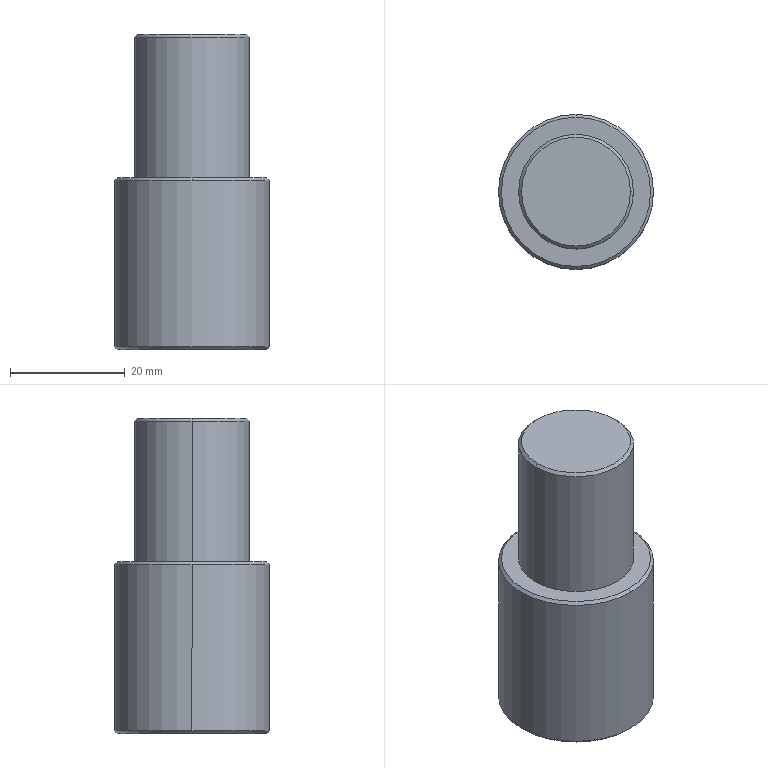Part | STEP file | Fixed head | 1 solid | 13 faces | box 27 x 27 x 55 mm | volume 25002 mm3 | cone 6 | cylinder 4 | plane 3 | commonest cylinder face diameters 20 x2 27 x2
STEP:
#1=CARTESIAN_POINT('',(0.,0.,0.));
#2=DIRECTION('',(0.,0.,1.));
#3=DIRECTION('',(1.,0.,0.));
#4=AXIS2_PLACEMENT_3D('',#1,#2,#3);
#5=CARTESIAN_POINT('',(0.,13.5,29.5));
#6=VERTEX_POINT('',#5);
#7=CARTESIAN_POINT('',(13.5,0.,29.5));
#8=VERTEX_POINT('',#7);
#9=CARTESIAN_POINT('',(0.,0.,29.5));
#10=DIRECTION('',(0.,0.,-1.));
#11=DIRECTION('',(-1.,0.,0.));
#12=AXIS2_PLACEMENT_3D('',#9,#10,#11);
#13=CIRCLE('',#12,13.5);
#14=CARTESIAN_POINT('',(0.,0.,30.));
#15=DIRECTION('',(0.,0.,-1.));
#16=DIRECTION('',(-1.,0.,0.));
#17=AXIS2_PLACEMENT_3D('',#14,#15,#16);
#18=CYLINDRICAL_SURFACE('',#17,13.5);
#19=CARTESIAN_POINT('',(0.,0.5));
#20=DIRECTION('',(1.,0.));
#21=VECTOR('',#20,1.);
#22=LINE('',#19,#21);
#23=(GEOMETRIC_REPRESENTATION_CONTEXT(2)PARAMETRIC_REPRESENTATION_CONTEXT()REPRESENTATION_CONTEXT('',''));
#24=DEFINITIONAL_REPRESENTATION('',(#22),#23);
#25=PCURVE('',#18,#24);
#26=CARTESIAN_POINT('',(0.,0.,29.5));
#27=DIRECTION('',(0.,0.,-1.));
#28=DIRECTION('',(0.,1.,0.));
#29=AXIS2_PLACEMENT_3D('',#26,#27,#28);
#30=CONICAL_SURFACE('',#29,13.5,0.7854);
#31=CARTESIAN_POINT('',(-1.571,0.));
#32=DIRECTION('',(1.,0.));
#33=VECTOR('',#32,1.);
#34=LINE('',#31,#33);
#35=(GEOMETRIC_REPRESENTATION_CONTEXT(2)PARAMETRIC_REPRESENTATION_CONTEXT()REPRESENTATION_CONTEXT('',''));
#36=DEFINITIONAL_REPRESENTATION('',(#34),#35);
#37=PCURVE('',#30,#36);
#38=SURFACE_CURVE('',#13,(#25,#37),.PCURVE_S1.);
#39=EDGE_CURVE('',#6,#8,#38,.T.);
#40=ORIENTED_EDGE('',*,*,#39,.T.);
#41=CARTESIAN_POINT('',(13.5,0.,0.5));
#42=VERTEX_POINT('',#41);
#43=CARTESIAN_POINT('',(13.5,0.,30.));
#44=DIRECTION('',(0.,0.,-1.));
#45=VECTOR('',#44,1.);
#46=LINE('',#43,#45);
#47=CARTESIAN_POINT('',(3.142,0.));
#48=DIRECTION('',(0.,1.));
#49=VECTOR('',#48,1.);
#50=LINE('',#47,#49);
#51=(GEOMETRIC_REPRESENTATION_CONTEXT(2)PARAMETRIC_REPRESENTATION_CONTEXT()REPRESENTATION_CONTEXT('',''));
#52=DEFINITIONAL_REPRESENTATION('',(#50),#51);
#53=PCURVE('',#18,#52);
#54=CARTESIAN_POINT('',(0.,0.,30.));
#55=DIRECTION('',(0.,0.,-1.));
#56=DIRECTION('',(-1.,0.,0.));
#57=AXIS2_PLACEMENT_3D('',#54,#55,#56);
#58=CYLINDRICAL_SURFACE('',#57,13.5);
#59=CARTESIAN_POINT('',(3.142,0.));
#60=DIRECTION('',(0.,1.));
#61=VECTOR('',#60,1.);
#62=LINE('',#59,#61);
#63=(GEOMETRIC_REPRESENTATION_CONTEXT(2)PARAMETRIC_REPRESENTATION_CONTEXT()REPRESENTATION_CONTEXT('',''));
#64=DEFINITIONAL_REPRESENTATION('',(#62),#63);
#65=PCURVE('',#58,#64);
#66=SURFACE_CURVE('',#46,(#53,#65),.PCURVE_S1.);
#67=EDGE_CURVE('',#8,#42,#66,.T.);
#68=ORIENTED_EDGE('',*,*,#67,.T.);
#69=CARTESIAN_POINT('',(-13.5,0.,0.5));
#70=VERTEX_POINT('',#69);
#71=CARTESIAN_POINT('',(0.,0.,0.5));
#72=DIRECTION('',(0.,0.,1.));
#73=DIRECTION('',(-1.,0.,0.));
#74=AXIS2_PLACEMENT_3D('',#71,#72,#73);
#75=CIRCLE('',#74,13.5);
#76=CARTESIAN_POINT('',(6.283,29.5));
#77=DIRECTION('',(-1.,0.));
#78=VECTOR('',#77,1.);
#79=LINE('',#76,#78);
#80=(GEOMETRIC_REPRESENTATION_CONTEXT(2)PARAMETRIC_REPRESENTATION_CONTEXT()REPRESENTATION_CONTEXT('',''));
#81=DEFINITIONAL_REPRESENTATION('',(#79),#80);
#82=PCURVE('',#18,#81);
#83=CARTESIAN_POINT('',(0.,0.,0.5));
#84=DIRECTION('',(0.,0.,1.));
#85=DIRECTION('',(1.,0.,0.));
#86=AXIS2_PLACEMENT_3D('',#83,#84,#85);
#87=CONICAL_SURFACE('',#86,13.5,0.7854);
#88=CARTESIAN_POINT('',(-3.142,0.));
#89=DIRECTION('',(1.,0.));
#90=VECTOR('',#89,1.);
#91=LINE('',#88,#90);
#92=(GEOMETRIC_REPRESENTATION_CONTEXT(2)PARAMETRIC_REPRESENTATION_CONTEXT()REPRESENTATION_CONTEXT('',''));
#93=DEFINITIONAL_REPRESENTATION('',(#91),#92);
#94=PCURVE('',#87,#93);
#95=SURFACE_CURVE('',#75,(#82,#94),.PCURVE_S1.);
#96=EDGE_CURVE('',#42,#70,#95,.T.);
#97=ORIENTED_EDGE('',*,*,#96,.T.);
#98=CARTESIAN_POINT('',(-13.5,0.,29.5));
#99=VERTEX_POINT('',#98);
#100=CARTESIAN_POINT('',(-13.5,0.,30.));
#101=DIRECTION('',(0.,0.,-1.));
#102=VECTOR('',#101,1.);
#103=LINE('',#100,#102);
#104=CARTESIAN_POINT('',(0.,0.));
#105=DIRECTION('',(0.,1.));
#106=VECTOR('',#105,1.);
#107=LINE('',#104,#106);
#108=(GEOMETRIC_REPRESENTATION_CONTEXT(2)PARAMETRIC_REPRESENTATION_CONTEXT()REPRESENTATION_CONTEXT('',''));
#109=DEFINITIONAL_REPRESENTATION('',(#107),#108);
#110=PCURVE('',#18,#109);
#111=CARTESIAN_POINT('',(6.283,0.));
#112=DIRECTION('',(0.,1.));
#113=VECTOR('',#112,1.);
#114=LINE('',#111,#113);
#115=(GEOMETRIC_REPRESENTATION_CONTEXT(2)PARAMETRIC_REPRESENTATION_CONTEXT()REPRESENTATION_CONTEXT('',''));
#116=DEFINITIONAL_REPRESENTATION('',(#114),#115);
#117=PCURVE('',#58,#116);
#118=SURFACE_CURVE('',#103,(#110,#117),.PCURVE_S1.);
#119=EDGE_CURVE('',#99,#70,#118,.T.);
#120=ORIENTED_EDGE('',*,*,#119,.F.);
#121=CARTESIAN_POINT('',(0.,0.,29.5));
#122=DIRECTION('',(0.,0.,-1.));
#123=DIRECTION('',(-1.,0.,0.));
#124=AXIS2_PLACEMENT_3D('',#121,#122,#123);
#125=CIRCLE('',#124,13.5);
#126=CARTESIAN_POINT('',(0.,0.5));
#127=DIRECTION('',(1.,0.));
#128=VECTOR('',#127,1.);
#129=LINE('',#126,#128);
#130=(GEOMETRIC_REPRESENTATION_CONTEXT(2)PARAMETRIC_REPRESENTATION_CONTEXT()REPRESENTATION_CONTEXT('',''));
#131=DEFINITIONAL_REPRESENTATION('',(#129),#130);
#132=PCURVE('',#18,#131);
#133=CARTESIAN_POINT('',(0.,0.,29.5));
#134=DIRECTION('',(0.,0.,-1.));
#135=DIRECTION('',(0.,1.,0.));
#136=AXIS2_PLACEMENT_3D('',#133,#134,#135);
#137=CONICAL_SURFACE('',#136,13.5,0.7854);
#138=CARTESIAN_POINT('',(4.712,0.));
#139=DIRECTION('',(1.,0.));
#140=VECTOR('',#139,1.);
#141=LINE('',#138,#140);
#142=(GEOMETRIC_REPRESENTATION_CONTEXT(2)PARAMETRIC_REPRESENTATION_CONTEXT()REPRESENTATION_CONTEXT('',''));
#143=DEFINITIONAL_REPRESENTATION('',(#141),#142);
#144=PCURVE('',#137,#143);
#145=SURFACE_CURVE('',#125,(#132,#144),.PCURVE_S1.);
#146=EDGE_CURVE('',#99,#6,#145,.T.);
#147=ORIENTED_EDGE('',*,*,#146,.T.);
#148=EDGE_LOOP('',(#40,#68,#97,#120,#147));
#149=FACE_BOUND('',#148,.T.);
#150=ADVANCED_FACE('',(#149),#18,.T.);
#151=CARTESIAN_POINT('',(13.,0.,0.));
#152=VERTEX_POINT('',#151);
#153=CARTESIAN_POINT('',(-13.,0.,0.));
#154=VERTEX_POINT('',#153);
#155=CARTESIAN_POINT('',(0.,0.,0.));
#156=DIRECTION('',(0.,0.,1.));
#157=DIRECTION('',(1.,0.,0.));
#158=AXIS2_PLACEMENT_3D('',#155,#156,#157);
#159=CIRCLE('',#158,13.);
#160=CARTESIAN_POINT('',(0.,-0.5));
#161=DIRECTION('',(1.,0.));
#162=VECTOR('',#161,1.);
#163=LINE('',#160,#162);
#164=(GEOMETRIC_REPRESENTATION_CONTEXT(2)PARAMETRIC_REPRESENTATION_CONTEXT()REPRESENTATION_CONTEXT('',''));
#165=DEFINITIONAL_REPRESENTATION('',(#163),#164);
#166=PCURVE('',#87,#165);
#167=CARTESIAN_POINT('',(0.,0.,0.));
#168=DIRECTION('',(0.,0.,1.));
#169=DIRECTION('',(1.,0.,0.));
#170=AXIS2_PLACEMENT_3D('',#167,#168,#169);
#171=PLANE('',#170);
#172=CARTESIAN_POINT('',(0.,0.));
#173=DIRECTION('',(1.,0.));
#174=AXIS2_PLACEMENT_2D('',#172,#173);
#175=CIRCLE('',#174,13.);
#176=(GEOMETRIC_REPRESENTATION_CONTEXT(2)PARAMETRIC_REPRESENTATION_CONTEXT()REPRESENTATION_CONTEXT('',''));
#177=DEFINITIONAL_REPRESENTATION('',(#175),#176);
#178=PCURVE('',#171,#177);
#179=SURFACE_CURVE('',#159,(#166,#178),.PCURVE_S1.);
#180=EDGE_CURVE('',#152,#154,#179,.T.);
#181=ORIENTED_EDGE('',*,*,#180,.T.);
#182=CARTESIAN_POINT('',(-13.5,0.,0.5));
#183=DIRECTION('',(-0.7071,0.,0.7071));
#184=VECTOR('',#183,1.);
#185=LINE('',#182,#184);
#186=CARTESIAN_POINT('',(3.142,0.));
#187=DIRECTION('',(0.,1.));
#188=VECTOR('',#187,1.);
#189=LINE('',#186,#188);
#190=(GEOMETRIC_REPRESENTATION_CONTEXT(2)PARAMETRIC_REPRESENTATION_CONTEXT()REPRESENTATION_CONTEXT('',''));
#191=DEFINITIONAL_REPRESENTATION('',(#189),#190);
#192=PCURVE('',#87,#191);
#193=CARTESIAN_POINT('',(0.,0.,0.5));
#194=DIRECTION('',(0.,0.,1.));
#195=DIRECTION('',(1.,0.,0.));
#196=AXIS2_PLACEMENT_3D('',#193,#194,#195);
#197=CONICAL_SURFACE('',#196,13.5,0.7854);
#198=CARTESIAN_POINT('',(3.142,0.));
#199=DIRECTION('',(0.,1.));
#200=VECTOR('',#199,1.);
#201=LINE('',#198,#200);
#202=(GEOMETRIC_REPRESENTATION_CONTEXT(2)PARAMETRIC_REPRESENTATION_CONTEXT()REPRESENTATION_CONTEXT('',''));
#203=DEFINITIONAL_REPRESENTATION('',(#201),#202);
#204=PCURVE('',#197,#203);
#205=SURFACE_CURVE('',#185,(#192,#204),.PCURVE_S1.);
#206=EDGE_CURVE('',#154,#70,#205,.T.);
#207=ORIENTED_EDGE('',*,*,#206,.T.);
#208=ORIENTED_EDGE('',*,*,#96,.F.);
#209=CARTESIAN_POINT('',(13.5,0.,0.5));
#210=DIRECTION('',(0.7071,0.,0.7071));
#211=VECTOR('',#210,1.);
#212=LINE('',#209,#211);
#213=CARTESIAN_POINT('',(0.,0.));
#214=DIRECTION('',(0.,1.));
#215=VECTOR('',#214,1.);
#216=LINE('',#213,#215);
#217=(GEOMETRIC_REPRESENTATION_CONTEXT(2)PARAMETRIC_REPRESENTATION_CONTEXT()REPRESENTATION_CONTEXT('',''));
#218=DEFINITIONAL_REPRESENTATION('',(#216),#217);
#219=PCURVE('',#87,#218);
#220=CARTESIAN_POINT('',(6.283,0.));
#221=DIRECTION('',(0.,1.));
#222=VECTOR('',#221,1.);
#223=LINE('',#220,#222);
#224=(GEOMETRIC_REPRESENTATION_CONTEXT(2)PARAMETRIC_REPRESENTATION_CONTEXT()REPRESENTATION_CONTEXT('',''));
#225=DEFINITIONAL_REPRESENTATION('',(#223),#224);
#226=PCURVE('',#197,#225);
#227=SURFACE_CURVE('',#212,(#219,#226),.PCURVE_S1.);
#228=EDGE_CURVE('',#152,#42,#227,.T.);
#229=ORIENTED_EDGE('',*,*,#228,.F.);
#230=EDGE_LOOP('',(#181,#207,#208,#229));
#231=FACE_BOUND('',#230,.T.);
#232=ADVANCED_FACE('',(#231),#87,.T.);
#233=CARTESIAN_POINT('',(0.,13.,30.));
#234=VERTEX_POINT('',#233);
#235=CARTESIAN_POINT('',(0.,-13.,30.));
#236=VERTEX_POINT('',#235);
#237=CARTESIAN_POINT('',(0.,0.,30.));
#238=DIRECTION('',(0.,0.,-1.));
#239=DIRECTION('',(0.,1.,0.));
#240=AXIS2_PLACEMENT_3D('',#237,#238,#239);
#241=CIRCLE('',#240,13.);
#242=CARTESIAN_POINT('',(0.,-0.5));
#243=DIRECTION('',(1.,0.));
#244=VECTOR('',#243,1.);
#245=LINE('',#242,#244);
#246=(GEOMETRIC_REPRESENTATION_CONTEXT(2)PARAMETRIC_REPRESENTATION_CONTEXT()REPRESENTATION_CONTEXT('',''));
#247=DEFINITIONAL_REPRESENTATION('',(#245),#246);
#248=PCURVE('',#30,#247);
#249=CARTESIAN_POINT('',(0.,0.,30.));
#250=DIRECTION('',(0.,0.,1.));
#251=DIRECTION('',(1.,0.,0.));
#252=AXIS2_PLACEMENT_3D('',#249,#250,#251);
#253=PLANE('',#252);
#254=CARTESIAN_POINT('',(0.,13.));
#255=CARTESIAN_POINT('',(22.517,13.));
#256=CARTESIAN_POINT('',(11.258,-6.5));
#257=CARTESIAN_POINT('',(0.,-26.));
#258=CARTESIAN_POINT('',(-11.258,-6.5));
#259=CARTESIAN_POINT('',(-22.517,13.));
#260=CARTESIAN_POINT('',(0.,13.));
#261=(BOUNDED_CURVE()B_SPLINE_CURVE(2,(#254,#255,#256,#257,#258,#259,#260),.UNSPECIFIED.,.T.,.F.)B_SPLINE_CURVE_WITH_KNOTS((1,2,2,2,2,1),(-2.094,0.,2.094,4.189,6.283,8.378),.UNSPECIFIED.)CURVE()GEOMETRIC_REPRESENTATION_ITEM()RATIONAL_B_SPLINE_CURVE((1.,0.5,1.,0.5,1.,0.5,1.))REPRESENTATION_ITEM(''));
#262=(GEOMETRIC_REPRESENTATION_CONTEXT(2)PARAMETRIC_REPRESENTATION_CONTEXT()REPRESENTATION_CONTEXT('',''));
#263=DEFINITIONAL_REPRESENTATION('',(#261),#262);
#264=PCURVE('',#253,#263);
#265=SURFACE_CURVE('',#241,(#248,#264),.PCURVE_S1.);
#266=EDGE_CURVE('',#234,#236,#265,.T.);
#267=ORIENTED_EDGE('',*,*,#266,.T.);
#268=CARTESIAN_POINT('',(0.,-13.5,29.5));
#269=VERTEX_POINT('',#268);
#270=CARTESIAN_POINT('',(0.,-13.5,29.5));
#271=DIRECTION('',(0.,-0.7071,-0.7071));
#272=VECTOR('',#271,1.);
#273=LINE('',#270,#272);
#274=CARTESIAN_POINT('',(3.142,0.));
#275=DIRECTION('',(0.,1.));
#276=VECTOR('',#275,1.);
#277=LINE('',#274,#276);
#278=(GEOMETRIC_REPRESENTATION_CONTEXT(2)PARAMETRIC_REPRESENTATION_CONTEXT()REPRESENTATION_CONTEXT('',''));
#279=DEFINITIONAL_REPRESENTATION('',(#277),#278);
#280=PCURVE('',#30,#279);
#281=CARTESIAN_POINT('',(3.142,0.));
#282=DIRECTION('',(0.,1.));
#283=VECTOR('',#282,1.);
#284=LINE('',#281,#283);
#285=(GEOMETRIC_REPRESENTATION_CONTEXT(2)PARAMETRIC_REPRESENTATION_CONTEXT()REPRESENTATION_CONTEXT('',''));
#286=DEFINITIONAL_REPRESENTATION('',(#284),#285);
#287=PCURVE('',#137,#286);
#288=SURFACE_CURVE('',#273,(#280,#287),.PCURVE_S1.);
#289=EDGE_CURVE('',#236,#269,#288,.T.);
#290=ORIENTED_EDGE('',*,*,#289,.T.);
#291=CARTESIAN_POINT('',(0.,0.,29.5));
#292=DIRECTION('',(0.,0.,-1.));
#293=DIRECTION('',(-1.,0.,0.));
#294=AXIS2_PLACEMENT_3D('',#291,#292,#293);
#295=CIRCLE('',#294,13.5);
#296=CARTESIAN_POINT('',(-1.571,0.));
#297=DIRECTION('',(1.,0.));
#298=VECTOR('',#297,1.);
#299=LINE('',#296,#298);
#300=(GEOMETRIC_REPRESENTATION_CONTEXT(2)PARAMETRIC_REPRESENTATION_CONTEXT()REPRESENTATION_CONTEXT('',''));
#301=DEFINITIONAL_REPRESENTATION('',(#299),#300);
#302=PCURVE('',#30,#301);
#303=CARTESIAN_POINT('',(0.,0.5));
#304=DIRECTION('',(1.,0.));
#305=VECTOR('',#304,1.);
#306=LINE('',#303,#305);
#307=(GEOMETRIC_REPRESENTATION_CONTEXT(2)PARAMETRIC_REPRESENTATION_CONTEXT()REPRESENTATION_CONTEXT('',''));
#308=DEFINITIONAL_REPRESENTATION('',(#306),#307);
#309=PCURVE('',#58,#308);
#310=SURFACE_CURVE('',#295,(#302,#309),.PCURVE_S1.);
#311=EDGE_CURVE('',#8,#269,#310,.T.);
#312=ORIENTED_EDGE('',*,*,#311,.F.);
#313=ORIENTED_EDGE('',*,*,#39,.F.);
#314=CARTESIAN_POINT('',(0.,13.5,29.5));
#315=DIRECTION('',(0.,0.7071,-0.7071));
#316=VECTOR('',#315,1.);
#317=LINE('',#314,#316);
#318=CARTESIAN_POINT('',(0.,0.));
#319=DIRECTION('',(0.,1.));
#320=VECTOR('',#319,1.);
#321=LINE('',#318,#320);
#322=(GEOMETRIC_REPRESENTATION_CONTEXT(2)PARAMETRIC_REPRESENTATION_CONTEXT()REPRESENTATION_CONTEXT('',''));
#323=DEFINITIONAL_REPRESENTATION('',(#321),#322);
#324=PCURVE('',#30,#323);
#325=CARTESIAN_POINT('',(6.283,0.));
#326=DIRECTION('',(0.,1.));
#327=VECTOR('',#326,1.);
#328=LINE('',#325,#327);
#329=(GEOMETRIC_REPRESENTATION_CONTEXT(2)PARAMETRIC_REPRESENTATION_CONTEXT()REPRESENTATION_CONTEXT('',''));
#330=DEFINITIONAL_REPRESENTATION('',(#328),#329);
#331=PCURVE('',#137,#330);
#332=SURFACE_CURVE('',#317,(#324,#331),.PCURVE_S1.);
#333=EDGE_CURVE('',#234,#6,#332,.T.);
#334=ORIENTED_EDGE('',*,*,#333,.F.);
#335=EDGE_LOOP('',(#267,#290,#312,#313,#334));
#336=FACE_BOUND('',#335,.T.);
#337=ADVANCED_FACE('',(#336),#30,.T.);
#338=CARTESIAN_POINT('',(-10.,0.,54.5));
#339=VERTEX_POINT('',#338);
#340=CARTESIAN_POINT('',(10.,0.,54.5));
#341=VERTEX_POINT('',#340);
#342=CARTESIAN_POINT('',(0.,0.,54.5));
#343=DIRECTION('',(0.,0.,-1.));
#344=DIRECTION('',(-1.,0.,0.));
#345=AXIS2_PLACEMENT_3D('',#342,#343,#344);
#346=CIRCLE('',#345,10.);
#347=CARTESIAN_POINT('',(0.,0.,55.));
#348=DIRECTION('',(0.,0.,-1.));
#349=DIRECTION('',(-1.,0.,0.));
#350=AXIS2_PLACEMENT_3D('',#347,#348,#349);
#351=CYLINDRICAL_SURFACE('',#350,10.);
#352=CARTESIAN_POINT('',(0.,0.5));
#353=DIRECTION('',(1.,0.));
#354=VECTOR('',#353,1.);
#355=LINE('',#352,#354);
#356=(GEOMETRIC_REPRESENTATION_CONTEXT(2)PARAMETRIC_REPRESENTATION_CONTEXT()REPRESENTATION_CONTEXT('',''));
#357=DEFINITIONAL_REPRESENTATION('',(#355),#356);
#358=PCURVE('',#351,#357);
#359=CARTESIAN_POINT('',(0.,0.,54.5));
#360=DIRECTION('',(0.,0.,-1.));
#361=DIRECTION('',(-1.,0.,0.));
#362=AXIS2_PLACEMENT_3D('',#359,#360,#361);
#363=CONICAL_SURFACE('',#362,10.,0.7854);
#364=CARTESIAN_POINT('',(0.,0.));
#365=DIRECTION('',(1.,0.));
#366=VECTOR('',#365,1.);
#367=LINE('',#364,#366);
#368=(GEOMETRIC_REPRESENTATION_CONTEXT(2)PARAMETRIC_REPRESENTATION_CONTEXT()REPRESENTATION_CONTEXT('',''));
#369=DEFINITIONAL_REPRESENTATION('',(#367),#368);
#370=PCURVE('',#363,#369);
#371=SURFACE_CURVE('',#346,(#358,#370),.PCURVE_S1.);
#372=EDGE_CURVE('',#339,#341,#371,.T.);
#373=ORIENTED_EDGE('',*,*,#372,.T.);
#374=CARTESIAN_POINT('',(10.,0.,30.));
#375=VERTEX_POINT('',#374);
#376=CARTESIAN_POINT('',(10.,0.,55.));
#377=DIRECTION('',(0.,0.,-1.));
#378=VECTOR('',#377,1.);
#379=LINE('',#376,#378);
#380=CARTESIAN_POINT('',(3.142,0.));
#381=DIRECTION('',(0.,1.));
#382=VECTOR('',#381,1.);
#383=LINE('',#380,#382);
#384=(GEOMETRIC_REPRESENTATION_CONTEXT(2)PARAMETRIC_REPRESENTATION_CONTEXT()REPRESENTATION_CONTEXT('',''));
#385=DEFINITIONAL_REPRESENTATION('',(#383),#384);
#386=PCURVE('',#351,#385);
#387=CARTESIAN_POINT('',(0.,0.,55.));
#388=DIRECTION('',(0.,0.,-1.));
#389=DIRECTION('',(-1.,0.,0.));
#390=AXIS2_PLACEMENT_3D('',#387,#388,#389);
#391=CYLINDRICAL_SURFACE('',#390,10.);
#392=CARTESIAN_POINT('',(3.142,0.));
#393=DIRECTION('',(0.,1.));
#394=VECTOR('',#393,1.);
#395=LINE('',#392,#394);
#396=(GEOMETRIC_REPRESENTATION_CONTEXT(2)PARAMETRIC_REPRESENTATION_CONTEXT()REPRESENTATION_CONTEXT('',''));
#397=DEFINITIONAL_REPRESENTATION('',(#395),#396);
#398=PCURVE('',#391,#397);
#399=SURFACE_CURVE('',#379,(#386,#398),.PCURVE_S1.);
#400=EDGE_CURVE('',#341,#375,#399,.T.);
#401=ORIENTED_EDGE('',*,*,#400,.T.);
#402=CARTESIAN_POINT('',(-10.,0.,30.));
#403=VERTEX_POINT('',#402);
#404=CARTESIAN_POINT('',(0.,0.,30.));
#405=DIRECTION('',(0.,0.,-1.));
#406=DIRECTION('',(-1.,0.,0.));
#407=AXIS2_PLACEMENT_3D('',#404,#405,#406);
#408=CIRCLE('',#407,10.);
#409=CARTESIAN_POINT('',(0.,25.));
#410=DIRECTION('',(1.,0.));
#411=VECTOR('',#410,1.);
#412=LINE('',#409,#411);
#413=(GEOMETRIC_REPRESENTATION_CONTEXT(2)PARAMETRIC_REPRESENTATION_CONTEXT()REPRESENTATION_CONTEXT('',''));
#414=DEFINITIONAL_REPRESENTATION('',(#412),#413);
#415=PCURVE('',#351,#414);
#416=CARTESIAN_POINT('',(-10.,0.));
#417=CARTESIAN_POINT('',(-10.,17.321));
#418=CARTESIAN_POINT('',(5.,8.66));
#419=CARTESIAN_POINT('',(20.,0.));
#420=CARTESIAN_POINT('',(5.,-8.66));
#421=CARTESIAN_POINT('',(-10.,-17.321));
#422=CARTESIAN_POINT('',(-10.,0.));
#423=(BOUNDED_CURVE()B_SPLINE_CURVE(2,(#416,#417,#418,#419,#420,#421,#422),.UNSPECIFIED.,.T.,.F.)B_SPLINE_CURVE_WITH_KNOTS((1,2,2,2,2,1),(-2.094,0.,2.094,4.189,6.283,8.378),.UNSPECIFIED.)CURVE()GEOMETRIC_REPRESENTATION_ITEM()RATIONAL_B_SPLINE_CURVE((1.,0.5,1.,0.5,1.,0.5,1.))REPRESENTATION_ITEM(''));
#424=(GEOMETRIC_REPRESENTATION_CONTEXT(2)PARAMETRIC_REPRESENTATION_CONTEXT()REPRESENTATION_CONTEXT('',''));
#425=DEFINITIONAL_REPRESENTATION('',(#423),#424);
#426=PCURVE('',#253,#425);
#427=SURFACE_CURVE('',#408,(#415,#426),.PCURVE_S1.);
#428=EDGE_CURVE('',#403,#375,#427,.T.);
#429=ORIENTED_EDGE('',*,*,#428,.F.);
#430=CARTESIAN_POINT('',(-10.,0.,55.));
#431=DIRECTION('',(0.,0.,-1.));
#432=VECTOR('',#431,1.);
#433=LINE('',#430,#432);
#434=CARTESIAN_POINT('',(0.,0.));
#435=DIRECTION('',(0.,1.));
#436=VECTOR('',#435,1.);
#437=LINE('',#434,#436);
#438=(GEOMETRIC_REPRESENTATION_CONTEXT(2)PARAMETRIC_REPRESENTATION_CONTEXT()REPRESENTATION_CONTEXT('',''));
#439=DEFINITIONAL_REPRESENTATION('',(#437),#438);
#440=PCURVE('',#351,#439);
#441=CARTESIAN_POINT('',(6.283,0.));
#442=DIRECTION('',(0.,1.));
#443=VECTOR('',#442,1.);
#444=LINE('',#441,#443);
#445=(GEOMETRIC_REPRESENTATION_CONTEXT(2)PARAMETRIC_REPRESENTATION_CONTEXT()REPRESENTATION_CONTEXT('',''));
#446=DEFINITIONAL_REPRESENTATION('',(#444),#445);
#447=PCURVE('',#391,#446);
#448=SURFACE_CURVE('',#433,(#440,#447),.PCURVE_S1.);
#449=EDGE_CURVE('',#339,#403,#448,.T.);
#450=ORIENTED_EDGE('',*,*,#449,.F.);
#451=EDGE_LOOP('',(#373,#401,#429,#450));
#452=FACE_BOUND('',#451,.T.);
#453=ADVANCED_FACE('',(#452),#351,.T.);
#454=CARTESIAN_POINT('',(-9.5,0.,55.));
#455=VERTEX_POINT('',#454);
#456=CARTESIAN_POINT('',(9.5,0.,55.));
#457=VERTEX_POINT('',#456);
#458=CARTESIAN_POINT('',(0.,0.,55.));
#459=DIRECTION('',(0.,0.,-1.));
#460=DIRECTION('',(-1.,0.,0.));
#461=AXIS2_PLACEMENT_3D('',#458,#459,#460);
#462=CIRCLE('',#461,9.5);
#463=CARTESIAN_POINT('',(0.,-0.5));
#464=DIRECTION('',(1.,0.));
#465=VECTOR('',#464,1.);
#466=LINE('',#463,#465);
#467=(GEOMETRIC_REPRESENTATION_CONTEXT(2)PARAMETRIC_REPRESENTATION_CONTEXT()REPRESENTATION_CONTEXT('',''));
#468=DEFINITIONAL_REPRESENTATION('',(#466),#467);
#469=PCURVE('',#363,#468);
#470=CARTESIAN_POINT('',(0.,0.,55.));
#471=DIRECTION('',(0.,0.,1.));
#472=DIRECTION('',(1.,0.,0.));
#473=AXIS2_PLACEMENT_3D('',#470,#471,#472);
#474=PLANE('',#473);
#475=CARTESIAN_POINT('',(-9.5,0.));
#476=CARTESIAN_POINT('',(-9.5,16.454));
#477=CARTESIAN_POINT('',(4.75,8.227));
#478=CARTESIAN_POINT('',(19.,0.));
#479=CARTESIAN_POINT('',(4.75,-8.227));
#480=CARTESIAN_POINT('',(-9.5,-16.454));
#481=CARTESIAN_POINT('',(-9.5,0.));
#482=(BOUNDED_CURVE()B_SPLINE_CURVE(2,(#475,#476,#477,#478,#479,#480,#481),.UNSPECIFIED.,.T.,.F.)B_SPLINE_CURVE_WITH_KNOTS((1,2,2,2,2,1),(-2.094,0.,2.094,4.189,6.283,8.378),.UNSPECIFIED.)CURVE()GEOMETRIC_REPRESENTATION_ITEM()RATIONAL_B_SPLINE_CURVE((1.,0.5,1.,0.5,1.,0.5,1.))REPRESENTATION_ITEM(''));
#483=(GEOMETRIC_REPRESENTATION_CONTEXT(2)PARAMETRIC_REPRESENTATION_CONTEXT()REPRESENTATION_CONTEXT('',''));
#484=DEFINITIONAL_REPRESENTATION('',(#482),#483);
#485=PCURVE('',#474,#484);
#486=SURFACE_CURVE('',#462,(#469,#485),.PCURVE_S1.);
#487=EDGE_CURVE('',#455,#457,#486,.T.);
#488=ORIENTED_EDGE('',*,*,#487,.T.);
#489=CARTESIAN_POINT('',(10.,0.,54.5));
#490=DIRECTION('',(0.7071,0.,-0.7071));
#491=VECTOR('',#490,1.);
#492=LINE('',#489,#491);
#493=CARTESIAN_POINT('',(3.142,0.));
#494=DIRECTION('',(0.,1.));
#495=VECTOR('',#494,1.);
#496=LINE('',#493,#495);
#497=(GEOMETRIC_REPRESENTATION_CONTEXT(2)PARAMETRIC_REPRESENTATION_CONTEXT()REPRESENTATION_CONTEXT('',''));
#498=DEFINITIONAL_REPRESENTATION('',(#496),#497);
#499=PCURVE('',#363,#498);
#500=CARTESIAN_POINT('',(0.,0.,54.5));
#501=DIRECTION('',(0.,0.,-1.));
#502=DIRECTION('',(-1.,0.,0.));
#503=AXIS2_PLACEMENT_3D('',#500,#501,#502);
#504=CONICAL_SURFACE('',#503,10.,0.7854);
#505=CARTESIAN_POINT('',(3.142,0.));
#506=DIRECTION('',(0.,1.));
#507=VECTOR('',#506,1.);
#508=LINE('',#505,#507);
#509=(GEOMETRIC_REPRESENTATION_CONTEXT(2)PARAMETRIC_REPRESENTATION_CONTEXT()REPRESENTATION_CONTEXT('',''));
#510=DEFINITIONAL_REPRESENTATION('',(#508),#509);
#511=PCURVE('',#504,#510);
#512=SURFACE_CURVE('',#492,(#499,#511),.PCURVE_S1.);
#513=EDGE_CURVE('',#457,#341,#512,.T.);
#514=ORIENTED_EDGE('',*,*,#513,.T.);
#515=ORIENTED_EDGE('',*,*,#372,.F.);
#516=CARTESIAN_POINT('',(-10.,0.,54.5));
#517=DIRECTION('',(-0.7071,0.,-0.7071));
#518=VECTOR('',#517,1.);
#519=LINE('',#516,#518);
#520=CARTESIAN_POINT('',(0.,0.));
#521=DIRECTION('',(0.,1.));
#522=VECTOR('',#521,1.);
#523=LINE('',#520,#522);
#524=(GEOMETRIC_REPRESENTATION_CONTEXT(2)PARAMETRIC_REPRESENTATION_CONTEXT()REPRESENTATION_CONTEXT('',''));
#525=DEFINITIONAL_REPRESENTATION('',(#523),#524);
#526=PCURVE('',#363,#525);
#527=CARTESIAN_POINT('',(6.283,0.));
#528=DIRECTION('',(0.,1.));
#529=VECTOR('',#528,1.);
#530=LINE('',#527,#529);
#531=(GEOMETRIC_REPRESENTATION_CONTEXT(2)PARAMETRIC_REPRESENTATION_CONTEXT()REPRESENTATION_CONTEXT('',''));
#532=DEFINITIONAL_REPRESENTATION('',(#530),#531);
#533=PCURVE('',#504,#532);
#534=SURFACE_CURVE('',#519,(#526,#533),.PCURVE_S1.);
#535=EDGE_CURVE('',#455,#339,#534,.T.);
#536=ORIENTED_EDGE('',*,*,#535,.F.);
#537=EDGE_LOOP('',(#488,#514,#515,#536));
#538=FACE_BOUND('',#537,.T.);
#539=ADVANCED_FACE('',(#538),#363,.T.);
#540=ORIENTED_EDGE('',*,*,#67,.F.);
#541=ORIENTED_EDGE('',*,*,#311,.T.);
#542=CARTESIAN_POINT('',(0.,0.,29.5));
#543=DIRECTION('',(0.,0.,-1.));
#544=DIRECTION('',(-1.,0.,0.));
#545=AXIS2_PLACEMENT_3D('',#542,#543,#544);
#546=CIRCLE('',#545,13.5);
#547=CARTESIAN_POINT('',(0.,0.5));
#548=DIRECTION('',(1.,0.));
#549=VECTOR('',#548,1.);
#550=LINE('',#547,#549);
#551=(GEOMETRIC_REPRESENTATION_CONTEXT(2)PARAMETRIC_REPRESENTATION_CONTEXT()REPRESENTATION_CONTEXT('',''));
#552=DEFINITIONAL_REPRESENTATION('',(#550),#551);
#553=PCURVE('',#58,#552);
#554=CARTESIAN_POINT('',(-1.571,0.));
#555=DIRECTION('',(1.,0.));
#556=VECTOR('',#555,1.);
#557=LINE('',#554,#556);
#558=(GEOMETRIC_REPRESENTATION_CONTEXT(2)PARAMETRIC_REPRESENTATION_CONTEXT()REPRESENTATION_CONTEXT('',''));
#559=DEFINITIONAL_REPRESENTATION('',(#557),#558);
#560=PCURVE('',#137,#559);
#561=SURFACE_CURVE('',#546,(#553,#560),.PCURVE_S1.);
#562=EDGE_CURVE('',#269,#99,#561,.T.);
#563=ORIENTED_EDGE('',*,*,#562,.T.);
#564=ORIENTED_EDGE('',*,*,#119,.T.);
#565=CARTESIAN_POINT('',(0.,0.,0.5));
#566=DIRECTION('',(0.,0.,1.));
#567=DIRECTION('',(-1.,0.,0.));
#568=AXIS2_PLACEMENT_3D('',#565,#566,#567);
#569=CIRCLE('',#568,13.5);
#570=CARTESIAN_POINT('',(6.283,29.5));
#571=DIRECTION('',(-1.,0.));
#572=VECTOR('',#571,1.);
#573=LINE('',#570,#572);
#574=(GEOMETRIC_REPRESENTATION_CONTEXT(2)PARAMETRIC_REPRESENTATION_CONTEXT()REPRESENTATION_CONTEXT('',''));
#575=DEFINITIONAL_REPRESENTATION('',(#573),#574);
#576=PCURVE('',#58,#575);
#577=CARTESIAN_POINT('',(3.142,0.));
#578=DIRECTION('',(1.,0.));
#579=VECTOR('',#578,1.);
#580=LINE('',#577,#579);
#581=(GEOMETRIC_REPRESENTATION_CONTEXT(2)PARAMETRIC_REPRESENTATION_CONTEXT()REPRESENTATION_CONTEXT('',''));
#582=DEFINITIONAL_REPRESENTATION('',(#580),#581);
#583=PCURVE('',#197,#582);
#584=SURFACE_CURVE('',#569,(#576,#583),.PCURVE_S1.);
#585=EDGE_CURVE('',#70,#42,#584,.T.);
#586=ORIENTED_EDGE('',*,*,#585,.T.);
#587=EDGE_LOOP('',(#540,#541,#563,#564,#586));
#588=FACE_BOUND('',#587,.T.);
#589=ADVANCED_FACE('',(#588),#58,.T.);
#590=ORIENTED_EDGE('',*,*,#206,.F.);
#591=CARTESIAN_POINT('',(0.,0.,0.));
#592=DIRECTION('',(0.,0.,1.));
#593=DIRECTION('',(1.,0.,0.));
#594=AXIS2_PLACEMENT_3D('',#591,#592,#593);
#595=CIRCLE('',#594,13.);
#596=CARTESIAN_POINT('',(0.,-0.5));
#597=DIRECTION('',(1.,0.));
#598=VECTOR('',#597,1.);
#599=LINE('',#596,#598);
#600=(GEOMETRIC_REPRESENTATION_CONTEXT(2)PARAMETRIC_REPRESENTATION_CONTEXT()REPRESENTATION_CONTEXT('',''));
#601=DEFINITIONAL_REPRESENTATION('',(#599),#600);
#602=PCURVE('',#197,#601);
#603=CARTESIAN_POINT('',(0.,0.));
#604=DIRECTION('',(1.,0.));
#605=AXIS2_PLACEMENT_2D('',#603,#604);
#606=CIRCLE('',#605,13.);
#607=(GEOMETRIC_REPRESENTATION_CONTEXT(2)PARAMETRIC_REPRESENTATION_CONTEXT()REPRESENTATION_CONTEXT('',''));
#608=DEFINITIONAL_REPRESENTATION('',(#606),#607);
#609=PCURVE('',#171,#608);
#610=SURFACE_CURVE('',#595,(#602,#609),.PCURVE_S1.);
#611=EDGE_CURVE('',#154,#152,#610,.T.);
#612=ORIENTED_EDGE('',*,*,#611,.T.);
#613=ORIENTED_EDGE('',*,*,#228,.T.);
#614=ORIENTED_EDGE('',*,*,#585,.F.);
#615=EDGE_LOOP('',(#590,#612,#613,#614));
#616=FACE_BOUND('',#615,.T.);
#617=ADVANCED_FACE('',(#616),#197,.T.);
#618=ORIENTED_EDGE('',*,*,#289,.F.);
#619=CARTESIAN_POINT('',(0.,0.,30.));
#620=DIRECTION('',(0.,0.,-1.));
#621=DIRECTION('',(0.,1.,0.));
#622=AXIS2_PLACEMENT_3D('',#619,#620,#621);
#623=CIRCLE('',#622,13.);
#624=CARTESIAN_POINT('',(0.,-0.5));
#625=DIRECTION('',(1.,0.));
#626=VECTOR('',#625,1.);
#627=LINE('',#624,#626);
#628=(GEOMETRIC_REPRESENTATION_CONTEXT(2)PARAMETRIC_REPRESENTATION_CONTEXT()REPRESENTATION_CONTEXT('',''));
#629=DEFINITIONAL_REPRESENTATION('',(#627),#628);
#630=PCURVE('',#137,#629);
#631=CARTESIAN_POINT('',(0.,13.));
#632=CARTESIAN_POINT('',(22.517,13.));
#633=CARTESIAN_POINT('',(11.258,-6.5));
#634=CARTESIAN_POINT('',(0.,-26.));
#635=CARTESIAN_POINT('',(-11.258,-6.5));
#636=CARTESIAN_POINT('',(-22.517,13.));
#637=CARTESIAN_POINT('',(0.,13.));
#638=(BOUNDED_CURVE()B_SPLINE_CURVE(2,(#631,#632,#633,#634,#635,#636,#637),.UNSPECIFIED.,.T.,.F.)B_SPLINE_CURVE_WITH_KNOTS((1,2,2,2,2,1),(-2.094,0.,2.094,4.189,6.283,8.378),.UNSPECIFIED.)CURVE()GEOMETRIC_REPRESENTATION_ITEM()RATIONAL_B_SPLINE_CURVE((1.,0.5,1.,0.5,1.,0.5,1.))REPRESENTATION_ITEM(''));
#639=(GEOMETRIC_REPRESENTATION_CONTEXT(2)PARAMETRIC_REPRESENTATION_CONTEXT()REPRESENTATION_CONTEXT('',''));
#640=DEFINITIONAL_REPRESENTATION('',(#638),#639);
#641=PCURVE('',#253,#640);
#642=SURFACE_CURVE('',#623,(#630,#641),.PCURVE_S1.);
#643=EDGE_CURVE('',#236,#234,#642,.T.);
#644=ORIENTED_EDGE('',*,*,#643,.T.);
#645=ORIENTED_EDGE('',*,*,#333,.T.);
#646=ORIENTED_EDGE('',*,*,#146,.F.);
#647=ORIENTED_EDGE('',*,*,#562,.F.);
#648=EDGE_LOOP('',(#618,#644,#645,#646,#647));
#649=FACE_BOUND('',#648,.T.);
#650=ADVANCED_FACE('',(#649),#137,.T.);
#651=ORIENTED_EDGE('',*,*,#180,.F.);
#652=ORIENTED_EDGE('',*,*,#611,.F.);
#653=EDGE_LOOP('',(#651,#652));
#654=FACE_BOUND('',#653,.T.);
#655=ADVANCED_FACE('',(#654),#171,.F.);
#656=ORIENTED_EDGE('',*,*,#428,.T.);
#657=CARTESIAN_POINT('',(0.,0.,30.));
#658=DIRECTION('',(0.,0.,-1.));
#659=DIRECTION('',(-1.,0.,0.));
#660=AXIS2_PLACEMENT_3D('',#657,#658,#659);
#661=CIRCLE('',#660,10.);
#662=CARTESIAN_POINT('',(-10.,0.));
#663=CARTESIAN_POINT('',(-10.,17.321));
#664=CARTESIAN_POINT('',(5.,8.66));
#665=CARTESIAN_POINT('',(20.,0.));
#666=CARTESIAN_POINT('',(5.,-8.66));
#667=CARTESIAN_POINT('',(-10.,-17.321));
#668=CARTESIAN_POINT('',(-10.,0.));
#669=(BOUNDED_CURVE()B_SPLINE_CURVE(2,(#662,#663,#664,#665,#666,#667,#668),.UNSPECIFIED.,.T.,.F.)B_SPLINE_CURVE_WITH_KNOTS((1,2,2,2,2,1),(-2.094,0.,2.094,4.189,6.283,8.378),.UNSPECIFIED.)CURVE()GEOMETRIC_REPRESENTATION_ITEM()RATIONAL_B_SPLINE_CURVE((1.,0.5,1.,0.5,1.,0.5,1.))REPRESENTATION_ITEM(''));
#670=(GEOMETRIC_REPRESENTATION_CONTEXT(2)PARAMETRIC_REPRESENTATION_CONTEXT()REPRESENTATION_CONTEXT('',''));
#671=DEFINITIONAL_REPRESENTATION('',(#669),#670);
#672=PCURVE('',#253,#671);
#673=CARTESIAN_POINT('',(0.,25.));
#674=DIRECTION('',(1.,0.));
#675=VECTOR('',#674,1.);
#676=LINE('',#673,#675);
#677=(GEOMETRIC_REPRESENTATION_CONTEXT(2)PARAMETRIC_REPRESENTATION_CONTEXT()REPRESENTATION_CONTEXT('',''));
#678=DEFINITIONAL_REPRESENTATION('',(#676),#677);
#679=PCURVE('',#391,#678);
#680=SURFACE_CURVE('',#661,(#672,#679),.PCURVE_S1.);
#681=EDGE_CURVE('',#375,#403,#680,.T.);
#682=ORIENTED_EDGE('',*,*,#681,.T.);
#683=EDGE_LOOP('',(#656,#682));
#684=FACE_BOUND('',#683,.T.);
#685=ORIENTED_EDGE('',*,*,#266,.F.);
#686=ORIENTED_EDGE('',*,*,#643,.F.);
#687=EDGE_LOOP('',(#685,#686));
#688=FACE_BOUND('',#687,.T.);
#689=ADVANCED_FACE('',(#684,#688),#253,.T.);
#690=ORIENTED_EDGE('',*,*,#400,.F.);
#691=CARTESIAN_POINT('',(0.,0.,54.5));
#692=DIRECTION('',(0.,0.,-1.));
#693=DIRECTION('',(-1.,0.,0.));
#694=AXIS2_PLACEMENT_3D('',#691,#692,#693);
#695=CIRCLE('',#694,10.);
#696=CARTESIAN_POINT('',(0.,0.5));
#697=DIRECTION('',(1.,0.));
#698=VECTOR('',#697,1.);
#699=LINE('',#696,#698);
#700=(GEOMETRIC_REPRESENTATION_CONTEXT(2)PARAMETRIC_REPRESENTATION_CONTEXT()REPRESENTATION_CONTEXT('',''));
#701=DEFINITIONAL_REPRESENTATION('',(#699),#700);
#702=PCURVE('',#391,#701);
#703=CARTESIAN_POINT('',(0.,0.));
#704=DIRECTION('',(1.,0.));
#705=VECTOR('',#704,1.);
#706=LINE('',#703,#705);
#707=(GEOMETRIC_REPRESENTATION_CONTEXT(2)PARAMETRIC_REPRESENTATION_CONTEXT()REPRESENTATION_CONTEXT('',''));
#708=DEFINITIONAL_REPRESENTATION('',(#706),#707);
#709=PCURVE('',#504,#708);
#710=SURFACE_CURVE('',#695,(#702,#709),.PCURVE_S1.);
#711=EDGE_CURVE('',#341,#339,#710,.T.);
#712=ORIENTED_EDGE('',*,*,#711,.T.);
#713=ORIENTED_EDGE('',*,*,#449,.T.);
#714=ORIENTED_EDGE('',*,*,#681,.F.);
#715=EDGE_LOOP('',(#690,#712,#713,#714));
#716=FACE_BOUND('',#715,.T.);
#717=ADVANCED_FACE('',(#716),#391,.T.);
#718=ORIENTED_EDGE('',*,*,#513,.F.);
#719=CARTESIAN_POINT('',(0.,0.,55.));
#720=DIRECTION('',(0.,0.,-1.));
#721=DIRECTION('',(-1.,0.,0.));
#722=AXIS2_PLACEMENT_3D('',#719,#720,#721);
#723=CIRCLE('',#722,9.5);
#724=CARTESIAN_POINT('',(0.,-0.5));
#725=DIRECTION('',(1.,0.));
#726=VECTOR('',#725,1.);
#727=LINE('',#724,#726);
#728=(GEOMETRIC_REPRESENTATION_CONTEXT(2)PARAMETRIC_REPRESENTATION_CONTEXT()REPRESENTATION_CONTEXT('',''));
#729=DEFINITIONAL_REPRESENTATION('',(#727),#728);
#730=PCURVE('',#504,#729);
#731=CARTESIAN_POINT('',(-9.5,0.));
#732=CARTESIAN_POINT('',(-9.5,16.454));
#733=CARTESIAN_POINT('',(4.75,8.227));
#734=CARTESIAN_POINT('',(19.,0.));
#735=CARTESIAN_POINT('',(4.75,-8.227));
#736=CARTESIAN_POINT('',(-9.5,-16.454));
#737=CARTESIAN_POINT('',(-9.5,0.));
#738=(BOUNDED_CURVE()B_SPLINE_CURVE(2,(#731,#732,#733,#734,#735,#736,#737),.UNSPECIFIED.,.T.,.F.)B_SPLINE_CURVE_WITH_KNOTS((1,2,2,2,2,1),(-2.094,0.,2.094,4.189,6.283,8.378),.UNSPECIFIED.)CURVE()GEOMETRIC_REPRESENTATION_ITEM()RATIONAL_B_SPLINE_CURVE((1.,0.5,1.,0.5,1.,0.5,1.))REPRESENTATION_ITEM(''));
#739=(GEOMETRIC_REPRESENTATION_CONTEXT(2)PARAMETRIC_REPRESENTATION_CONTEXT()REPRESENTATION_CONTEXT('',''));
#740=DEFINITIONAL_REPRESENTATION('',(#738),#739);
#741=PCURVE('',#474,#740);
#742=SURFACE_CURVE('',#723,(#730,#741),.PCURVE_S1.);
#743=EDGE_CURVE('',#457,#455,#742,.T.);
#744=ORIENTED_EDGE('',*,*,#743,.T.);
#745=ORIENTED_EDGE('',*,*,#535,.T.);
#746=ORIENTED_EDGE('',*,*,#711,.F.);
#747=EDGE_LOOP('',(#718,#744,#745,#746));
#748=FACE_BOUND('',#747,.T.);
#749=ADVANCED_FACE('',(#748),#504,.T.);
#750=ORIENTED_EDGE('',*,*,#487,.F.);
#751=ORIENTED_EDGE('',*,*,#743,.F.);
#752=EDGE_LOOP('',(#750,#751));
#753=FACE_BOUND('',#752,.T.);
#754=ADVANCED_FACE('',(#753),#474,.T.);
#755=CLOSED_SHELL('',(#150,#232,#337,#453,#539,#589,#617,#650,#655,#689,#717,#749,#754));
#756=MANIFOLD_SOLID_BREP('',#755);
#757=(LENGTH_UNIT()NAMED_UNIT(*)SI_UNIT(.MILLI.,.METRE.));
#758=UNCERTAINTY_MEASURE_WITH_UNIT(LENGTH_MEASURE(0.0000001),#757,'','');
#759=(NAMED_UNIT(*)PLANE_ANGLE_UNIT()SI_UNIT($,.RADIAN.));
#760=(NAMED_UNIT(*)SI_UNIT($,.STERADIAN.)SOLID_ANGLE_UNIT());
#761=(GEOMETRIC_REPRESENTATION_CONTEXT(3)GLOBAL_UNCERTAINTY_ASSIGNED_CONTEXT((#758))GLOBAL_UNIT_ASSIGNED_CONTEXT((#757,#759,#760))REPRESENTATION_CONTEXT('',''));
#762=ADVANCED_BREP_SHAPE_REPRESENTATION('',(#4,#756),#761);